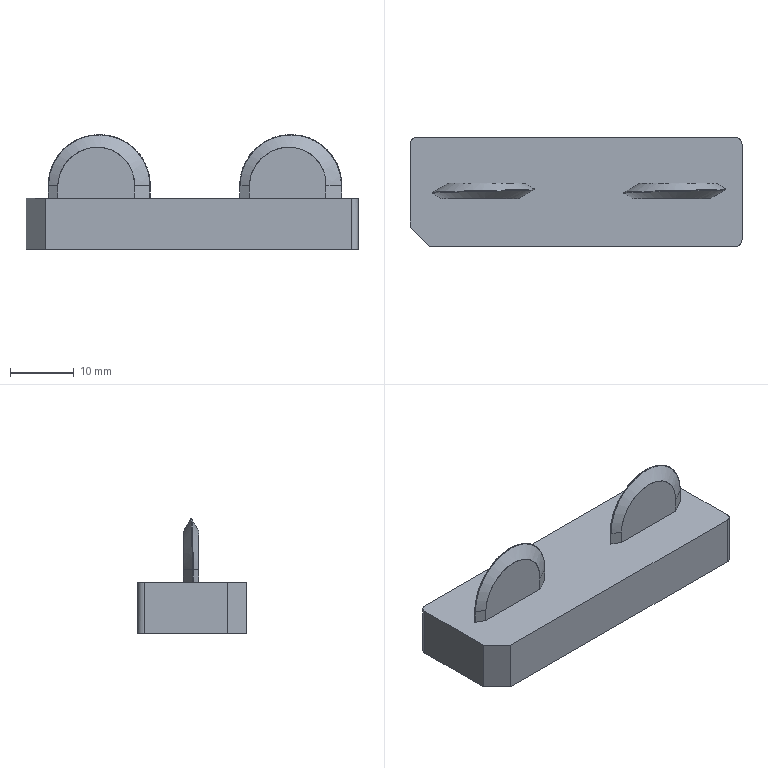NC program | PowerMill | posted with a generic post | part box 52 x 17 x 17.993 mm
Lines 10241 to 10969 of 175197:
N10338 M6
N10339 S18000 M03
N10340 G00 G90 X0.0 Y0.0
N10341 G43 Z10.802 H4
N10342
N10343 G05 P10000 R8
N10344 X-8.3293 Y-0.1432
N10345 Z-1.5814
N10346 G01 Z-2.7814 F1200.0
N10347 X-8.3275 Y-0.123 Z-2.802 F2000.0
N10348 X-8.3219 Y-0.1023 Z-2.8212
N10349 X-8.3129 Y-0.0816 Z-2.8384
N10350 X-8.3006 Y-0.0614 Z-2.8535
N10351 X-8.2852 Y-0.0419 Z-2.8662
N10352 X-8.2758 Y-0.032 Z-2.872
N10353 X-8.235 Y0.0088 Z-2.8945
N10354 X-8.1927 Y0.0511 Z-2.922
N10355 X-8.1485 Y0.0954 Z-2.955
N10356 X-8.1476 Y0.0962 Z-2.9557
N10357 X-8.1288 Y0.1132 Z-2.9682
N10358 X-8.1075 Y0.1291 Z-2.9777
N10359 X-8.0841 Y0.1435 Z-2.9842
N10360 X-8.0591 Y0.1563 Z-2.9874
N10361 X-8.033 Y0.1671
N10362 X-8.0181 Y0.1721 Z-2.9859
N10363 X-7.9685 Y0.2693 Z-3.0277
N10364 X-7.9946 Y0.2585 Z-3.0287
N10365 X-8.0198 Y0.246 Z-3.0263
N10366 X-8.0436 Y0.232 Z-3.0204
N10367 X-8.0655 Y0.2167 Z-3.0112
N10368 X-8.0851 Y0.2006 Z-2.9989
N10369 X-8.095 Y0.1913 Z-2.9908
N10370 X-8.12 Y0.1662 Z-2.9679
N10371 X-8.1518 Y0.1345 Z-2.941
N10372 X-8.1895 Y0.0967 Z-2.9117
N10373 X-8.2367 Y0.0495 Z-2.8782
N10374 X-8.2837 Y0.0026 Z-2.8484
N10375 X-8.3231 Y-0.0368 Z-2.8262
N10376 X-8.3579 Y-0.0716 Z-2.809
N10377 X-8.3933 Y-0.107 Z-2.7944
N10378 X-8.4111 Y-0.1269 Z-2.7853
N10379 X-8.426 Y-0.1479 Z-2.7737
N10380 X-8.4377 Y-0.1696 Z-2.7599
N10381 X-8.4459 Y-0.1915 Z-2.7441
N10382 X-8.4504 Y-0.2133 Z-2.7267
N10383 X-8.4514 Y-0.2252 Z-2.7164
N10384 X-8.5444 Y-0.2776 Z-2.6643
N10385 X-8.5416 Y-0.2552 Z-2.6813
N10386 X-8.535 Y-0.2325 Z-2.6968
N10387 X-8.525 Y-0.2099 Z-2.7104
N10388 X-8.5115 Y-0.188 Z-2.722
N10389 X-8.4951 Y-0.167 Z-2.7313
N10390 X-8.4846 Y-0.1559 Z-2.7354
N10391 X-8.4404 Y-0.1118 Z-2.7505
N10392 X-8.3948 Y-0.0661 Z-2.77
N10393 X-8.3471 Y-0.0184 Z-2.7943
N10394 X-8.2975 Y0.0312 Z-2.8237
N10395 X-8.2464 Y0.0823 Z-2.8582
N10396 X-8.1947 Y0.134 Z-2.8975
N10397 X-8.144 Y0.1847 Z-2.9403
N10398 X-8.097 Y0.2317 Z-2.9841
N10399 X-8.0804 Y0.2482 Z-3.0005
N10400 X-8.0627 Y0.2644 Z-3.0153
N10401 X-8.0424 Y0.2801 Z-3.0271
N10402 X-8.0199 Y0.2948 Z-3.0356
N10403 X-7.9957 Y0.3084 Z-3.0408
N10404 X-7.9703 Y0.3206 Z-3.0424
N10405 X-7.9557 Y0.3267 Z-3.0418
N10406 X-7.9564 Y0.371 Z-3.0433
N10407 X-7.982 Y0.3592 Z-3.0434
N10408 X-8.0067 Y0.3459 Z-3.0399
N10409 X-8.0299 Y0.3315 Z-3.0328
N10410 X-8.0513 Y0.3162 Z-3.0224
N10411 X-8.0703 Y0.3004 Z-3.0088
N10412 X-8.0797 Y0.2914 Z-2.9999
N10413 X-8.1111 Y0.2601 Z-2.9675
N10414 X-8.1603 Y0.2108 Z-2.9201
N10415 X-8.2121 Y0.1591 Z-2.8749
N10416 X-8.2643 Y0.1068 Z-2.8337
N10417 X-8.3161 Y0.055 Z-2.7971
N10418 X-8.3667 Y0.0044 Z-2.7656
N10419 X-8.416 Y-0.0449 Z-2.7389
N10420 X-8.4637 Y-0.0926 Z-2.7171
N10421 X-8.5098 Y-0.1386 Z-2.6998
N10422 X-8.5543 Y-0.1832 Z-2.687
N10423 X-8.5726 Y-0.2036 Z-2.68
N10424 X-8.588 Y-0.2253 Z-2.6707
N10425 X-8.6002 Y-0.248 Z-2.6591
N10426 X-8.609 Y-0.2711 Z-2.6455
N10427 X-8.6143 Y-0.2942 Z-2.6302
N10428 X-8.6156 Y-0.307 Z-2.621
N10429 X-8.6837 Y-0.3327 Z-2.583
N10430 X-8.68 Y-0.3093 Z-2.5983
N10431 X-8.6728 Y-0.2857 Z-2.6119
N10432 X-8.662 Y-0.2623 Z-2.6235
N10433 X-8.648 Y-0.2397 Z-2.6329
N10434 X-8.6311 Y-0.2182 Z-2.64
N10435 X-8.6204 Y-0.2069 Z-2.6428
N10436 X-8.5788 Y-0.1652 Z-2.6521
N10437 X-8.5355 Y-0.122 Z-2.6655
N10438 X-8.4902 Y-0.0767 Z-2.6835
N10439 X-8.4428 Y-0.0293 Z-2.7061
N10440 X-8.3934 Y0.0202 Z-2.7338
N10441 X-8.3421 Y0.0715 Z-2.7667
N10442 X-8.2894 Y0.1241 Z-2.8047
N10443 X-8.2365 Y0.1771 Z-2.8473
N10444 X-8.1856 Y0.228 Z-2.8926
N10445 X-8.1387 Y0.2748 Z-2.9381
N10446 X-8.0965 Y0.317 Z-2.9826
N10447 X-8.0855 Y0.328 Z-2.9949
N10448 X-8.0684 Y0.3437 Z-3.0109
N10449 X-8.0488 Y0.3593 Z-3.0239
N10450 X-8.0269 Y0.3743 Z-3.0336
N10451 X-8.0034 Y0.3886 Z-3.0398
N10452 X-7.9785 Y0.4017 Z-3.0423
N10453 X-7.9643 Y0.4085 Z-3.0422
N10454 X-7.9748 Y0.4434 Z-3.0362
N10455 X-7.9998 Y0.4303 Z-3.0356
N10456 X-8.0238 Y0.4162 Z-3.0313
N10457 X-8.0464 Y0.4012 Z-3.0233
N10458 X-8.0671 Y0.3857 Z-3.0119
N10459 X-8.0855 Y0.3701 Z-2.9973
N10460 X-8.0946 Y0.3614 Z-2.9878
N10461 X-8.1104 Y0.3456 Z-2.9698
N10462 X-8.153 Y0.3029 Z-2.9235
N10463 X-8.2003 Y0.2557 Z-2.8761
N10464 X-8.2515 Y0.2044 Z-2.8289
N10465 X-8.3049 Y0.1511 Z-2.7843
N10466 X-8.3581 Y0.0979 Z-2.7441
N10467 X-8.4102 Y0.0458 Z-2.7089
N10468 X-8.4607 Y-0.0047 Z-2.679
N10469 X-8.5093 Y-0.0534 Z-2.6541
N10470 X-8.5561 Y-0.1001 Z-2.634
N10471 X-8.601 Y-0.145 Z-2.6184
N10472 X-8.644 Y-0.188 Z-2.6073
N10473 X-8.6854 Y-0.2294 Z-2.6003
N10474 X-8.7039 Y-0.2501 Z-2.5956
N10475 X-8.7198 Y-0.2724 Z-2.5886
N10476 X-8.7326 Y-0.2957 Z-2.5791
N10477 X-8.7421 Y-0.3196 Z-2.5676
N10478 X-8.7481 Y-0.3437 Z-2.5541
N10479 X-8.7499 Y-0.3571 Z-2.5458
N10480 X-8.8128 Y-0.3782 Z-2.5117
N10481 X-8.8085 Y-0.3537 Z-2.5251
N10482 X-8.8006 Y-0.3292 Z-2.5366
N10483 X-8.7894 Y-0.305 Z-2.546
N10484 X-8.775 Y-0.2818 Z-2.5531
N10485 X-8.7577 Y-0.26 Z-2.5578
N10486 X-8.7469 Y-0.2485 Z-2.5594
N10487 X-8.714 Y-0.2156 Z-2.5628
N10488 X-8.6799 Y-0.1816 Z-2.5695
N10489 X-8.6408 Y-0.1424 Z-2.5803
N10490 X-8.5955 Y-0.0971 Z-2.5962
N10491 X-8.5466 Y-0.0482 Z-2.6171
N10492 X-8.5059 Y-0.0075 Z-2.6373
N10493 X-8.4721 Y0.0262 Z-2.6561
N10494 X-8.4418 Y0.0566 Z-2.6749
N10495 X-8.3885 Y0.1099 Z-2.7115
N10496 X-8.3346 Y0.1638 Z-2.753
N10497 X-8.2801 Y0.2183 Z-2.7994
N10498 X-8.2257 Y0.2727 Z-2.8503
N10499 X-8.1721 Y0.3263 Z-2.9051
N10500 X-8.1206 Y0.3778 Z-2.9626
N10501 X-8.106 Y0.3924 Z-2.9798
N10502 X-8.0893 Y0.4078 Z-2.9965
N10503 X-8.07 Y0.4232 Z-3.0101
N10504 X-8.0485 Y0.4384 Z-3.0205
N10505 X-8.0253 Y0.4529 Z-3.0272
N10506 X-8.0007 Y0.4665 Z-3.0304
N10507 X-7.9866 Y0.4737 Z-3.0305
N10508 X-8.0003 Y0.5045 Z-3.0226
N10509 X-8.0251 Y0.4911 Z-3.0216
N10510 X-8.0489 Y0.4767 Z-3.0169
N10511 X-8.0713 Y0.4616 Z-3.0085
N10512 X-8.0917 Y0.4462 Z-2.9966
N10513 X-8.1098 Y0.4306 Z-2.9816
N10514 X-8.1188 Y0.422 Z-2.9718
N10515 X-8.1632 Y0.3777 Z-2.9189
N10516 X-8.2114 Y0.3294 Z-2.8658
N10517 X-8.2661 Y0.2747 Z-2.8103
N10518 X-8.3181 Y0.2227 Z-2.7617
N10519 X-8.3704 Y0.1705 Z-2.7169
N10520 X-8.4067 Y0.1342 Z-2.6883
N10521 X-8.4475 Y0.0933 Z-2.6591
N10522 X-8.4939 Y0.0469 Z-2.6292
N10523 X-8.5451 Y-0.0043 Z-2.6
N10524 X-8.5962 Y-0.0554 Z-2.5749
N10525 X-8.6446 Y-0.1038 Z-2.5548
N10526 X-8.6897 Y-0.1489 Z-2.5398
N10527 X-8.7316 Y-0.1908 Z-2.5292
N10528 X-8.7704 Y-0.2295 Z-2.5229
N10529 X-8.8071 Y-0.2663 Z-2.5203
N10530 X-8.8259 Y-0.2872 Z-2.5176
N10531 X-8.842 Y-0.3098 Z-2.5124
N10532 X-8.8552 Y-0.3336 Z-2.5049
N10533 X-8.8652 Y-0.3581 Z-2.4951
N10534 X-8.8718 Y-0.3829 Z-2.4832
N10535 X-8.8739 Y-0.3967 Z-2.4758
N10536 X-8.9331 Y-0.4139 Z-2.4406
N10537 X-8.9284 Y-0.389 Z-2.453
N10538 X-8.9203 Y-0.3641 Z-2.4635
N10539 X-8.9088 Y-0.3397 Z-2.4719
N10540 X-8.8942 Y-0.3163 Z-2.4779
N10541 X-8.8769 Y-0.2943 Z-2.4815
N10542 X-8.8661 Y-0.2828 Z-2.4824
N10543 X-8.8245 Y-0.2413 Z-2.4844
N10544 X-8.782 Y-0.1987 Z-2.4903
N10545 X-8.738 Y-0.1547 Z-2.5003
N10546 X-8.6924 Y-0.1091 Z-2.5147
N10547 X-8.6449 Y-0.0616 Z-2.5336
N10548 X-8.595 Y-0.0117 Z-2.5575
N10549 X-8.5546 Y0.0286 Z-2.5796
N10550 X-8.502 Y0.0813 Z-2.612
N10551 X-8.4491 Y0.1341 Z-2.6489
N10552 X-8.396 Y0.1872 Z-2.6903
N10553 X-8.3427 Y0.2406 Z-2.7365
N10554 X-8.2891 Y0.2941 Z-2.7874
N10555 X-8.2353 Y0.3479 Z-2.8432
N10556 X-8.1814 Y0.4018 Z-2.9041
N10557 X-8.1293 Y0.4539 Z-2.9676
N10558 X-8.1129 Y0.4693 Z-2.9846
N10559 X-8.0939 Y0.4849 Z-2.9985
N10560 X-8.0729 Y0.5005 Z-3.009
N10561 X-8.0501 Y0.5158 Z-3.016
N10562 X-8.0262 Y0.5304 Z-3.0191
N10563 X-8.0124 Y0.5382 Z-3.0192
N10564 X-8.0264 Y0.5669 Z-3.0181
N10565 X-8.0507 Y0.5528 Z-3.0162
N10566 X-8.0741 Y0.5379 Z-3.0106
N10567 X-8.0959 Y0.5226 Z-3.0013
N10568 X-8.1158 Y0.5072 Z-2.9886
N10569 X-8.1333 Y0.492 Z-2.9726
N10570 X-8.1421 Y0.4836 Z-2.9623
N10571 X-8.157 Y0.4687 Z-2.943
N10572 X-8.2099 Y0.4158 Z-2.8779
N10573 X-8.2656 Y0.36 Z-2.8145
N10574 X-8.3071 Y0.3185 Z-2.7705
N10575 X-8.3497 Y0.2759 Z-2.7286
N10576 X-8.3933 Y0.2323 Z-2.6888
N10577 X-8.4462 Y0.1795 Z-2.6443
N10578 X-8.4917 Y0.1339 Z-2.6092
N10579 X-8.5383 Y0.0874 Z-2.5768
N10580 X-8.5882 Y0.0374 Z-2.5458
N10581 X-8.6389 Y-0.0133 Z-2.518
N10582 X-8.6873 Y-0.0616 Z-2.4954
N10583 X-8.7341 Y-0.1084 Z-2.4774
N10584 X-8.7806 Y-0.155 Z-2.4636
N10585 X-8.8277 Y-0.202 Z-2.4536
N10586 X-8.8752 Y-0.2495 Z-2.4477
N10587 X-8.9229 Y-0.2972 Z-2.4457
N10588 X-8.9417 Y-0.3182 Z-2.4436
N10589 X-8.9578 Y-0.3409 Z-2.439
N10590 X-8.9711 Y-0.3648 Z-2.4321
N10591 X-8.9811 Y-0.3896 Z-2.4229
N10592 X-8.9877 Y-0.4146 Z-2.4117
N10593 X-8.9899 Y-0.4286 Z-2.4046
N10594 X-9.0488 Y-0.4451 Z-2.3771
N10595 X-9.0437 Y-0.4197 Z-2.3881
N10596 X-9.0352 Y-0.3943 Z-2.3971
N10597 X-9.0234 Y-0.3695 Z-2.4039
N10598 X-9.0087 Y-0.3459 Z-2.4083
N10599 X-8.9912 Y-0.3238 Z-2.4102
N10600 X-8.9804 Y-0.3123
N10601 X-8.9432 Y-0.2751 Z-2.4088
N10602 X-8.9039 Y-0.2358 Z-2.4111
N10603 X-8.8618 Y-0.1937 Z-2.4173
N10604 X-8.8171 Y-0.149 Z-2.4278
N10605 X-8.7697 Y-0.1016 Z-2.4427
N10606 X-8.7198 Y-0.0517 Z-2.4624
N10607 X-8.6685 Y-0.0004 Z-2.4866
N10608 X-8.6182 Y0.0499 Z-2.5143
N10609 X-8.5722 Y0.0959 Z-2.5431
N10610 X-8.5319 Y0.1362 Z-2.5711
N10611 X-8.479 Y0.1891 Z-2.612
N10612 X-8.426 Y0.2421 Z-2.6573
N10613 X-8.3713 Y0.2968 Z-2.7084
N10614 X-8.3157 Y0.3524 Z-2.7651
N10615 X-8.2606 Y0.4075 Z-2.8261
N10616 X-8.209 Y0.4591 Z-2.888
N10617 X-8.1618 Y0.5063 Z-2.9491
N10618 X-8.1561 Y0.512 Z-2.9568
N10619 X-8.1403 Y0.5268 Z-2.9749
N10620 X-8.122 Y0.5422 Z-2.9899
N10621 X-8.1015 Y0.5577 Z-3.0016
N10622 X-8.0793 Y0.5732 Z-3.0097
N10623 X-8.0558 Y0.5882 Z-3.0141
N10624 X-8.0423 Y0.5964 Z-3.0148
N10625 X-8.0598 Y0.6245 Z-3.0064
N10626 X-8.0834 Y0.6091 Z-3.0043
N10627 X-8.1061 Y0.5934 Z-2.9985
N10628 X-8.1273 Y0.5774 Z-2.9889
N10629 X-8.1467 Y0.5617 Z-2.9758
N10630 X-8.1639 Y0.5464 Z-2.9594
N10631 X-8.1724 Y0.5381 Z-2.9489
N10632 X-8.2011 Y0.5095 Z-2.9102
N10633 X-8.2545 Y0.456 Z-2.842
N10634 X-8.309 Y0.4015 Z-2.7778
N10635 X-8.3639 Y0.3466 Z-2.7181
N10636 X-8.4188 Y0.2917 Z-2.6632
N10637 X-8.4733 Y0.2372 Z-2.6133
N10638 X-8.5273 Y0.1832 Z-2.5684
N10639 X-8.5807 Y0.1298 Z-2.5284
N10640 X-8.6178 Y0.0927 Z-2.5032
N10641 X-8.6675 Y0.043 Z-2.4728
N10642 X-8.7186 Y-0.0081 Z-2.4455
N10643 X-8.7692 Y-0.0587 Z-2.4223
N10644 X-8.8184 Y-0.1079 Z-2.4038
N10645 X-8.8658 Y-0.1552 Z-2.3897
N10646 X-8.9111 Y-0.2006 Z-2.3801
N10647 X-8.9544 Y-0.2439 Z-2.3746
N10648 X-8.9957 Y-0.2851 Z-2.373
N10649 X-9.035 Y-0.3244 Z-2.3753
N10650 X-9.0538 Y-0.3455 Z-2.3751
N10651 X-9.0701 Y-0.3683 Z-2.3725
N10652 X-9.0836 Y-0.3926 Z-2.3675
N10653 X-9.094 Y-0.4178 Z-2.3602
N10654 X-9.1011 Y-0.4434 Z-2.3506
N10655 X-9.1036 Y-0.4577 Z-2.3444
N10656 X-9.1582 Y-0.4699 Z-2.3159
N10657 X-9.1527 Y-0.444 Z-2.3257
N10658 X-9.1439 Y-0.4183 Z-2.3334
N10659 X-9.132 Y-0.3933 Z-2.3388
N10660 X-9.1171 Y-0.3695 Z-2.3417
N10661 X-9.0996 Y-0.3473 Z-2.3422
N10662 X-9.0888 Y-0.3358 Z-2.3413
N10663 X-9.0582 Y-0.3053 Z-2.3379
N10664 X-9.0266 Y-0.2737 Z-2.3374
N10665 X-8.9897 Y-0.2368 Z-2.3398
N10666 X-8.9464 Y-0.1935 Z-2.3459
N10667 X-8.8997 Y-0.1467 Z-2.3561
N10668 X-8.8604 Y-0.1074 Z-2.3674
N10669 X-8.8272 Y-0.0742 Z-2.3792
N10670 X-8.7777 Y-0.0248 Z-2.4004
N10671 X-8.727 Y0.0259 Z-2.4261
N10672 X-8.6746 Y0.0784 Z-2.4567
N10673 X-8.6208 Y0.1322 Z-2.4923
N10674 X-8.5662 Y0.1867 Z-2.5328
N10675 X-8.5119 Y0.241 Z-2.5775
N10676 X-8.4596 Y0.2933 Z-2.625
N10677 X-8.4091 Y0.3438 Z-2.6751
N10678 X-8.353 Y0.3999 Z-2.7353
N10679 X-8.2975 Y0.4555 Z-2.7998
N10680 X-8.2429 Y0.51 Z-2.8684
N10681 X-8.19 Y0.5629 Z-2.9401
N10682 X-8.189 Y0.5639 Z-2.9415
N10683 X-8.1735 Y0.5785 Z-2.9601
N10684 X-8.1556 Y0.5937 Z-2.9756
N10685 X-8.1354 Y0.6093 Z-2.9878
N10686 X-8.1136 Y0.625 Z-2.9964
N10687 X-8.0904 Y0.6404 Z-3.0012
N10688 X-8.077 Y0.6488 Z-3.0022
N10689 X-8.1 Y0.6716 Z-2.9892
N10690 X-8.1233 Y0.6558 Z-2.9867
N10691 X-8.1456 Y0.6398 Z-2.9803
N10692 X-8.1665 Y0.6237 Z-2.9702
N10693 X-8.1855 Y0.6079 Z-2.9566
N10694 X-8.2024 Y0.5928 Z-2.9397
N10695 X-8.2107 Y0.5847 Z-2.929
N10696 X-8.243 Y0.5524 Z-2.8834
N10697 X-8.2938 Y0.5016 Z-2.8159
N10698 X-8.347 Y0.4483 Z-2.7503
N10699 X-8.4016 Y0.3938 Z-2.6881
N10700 X-8.4567 Y0.3387 Z-2.6301
N10701 X-8.5119 Y0.2835 Z-2.5769
N10702 X-8.5667 Y0.2287 Z-2.5285
N10703 X-8.621 Y0.1744 Z-2.4852
N10704 X-8.6746 Y0.1208 Z-2.4467
N10705 X-8.7273 Y0.0681 Z-2.4131
N10706 X-8.7792 Y0.0162 Z-2.3841
N10707 X-8.8301 Y-0.0347 Z-2.3598
N10708 X-8.8801 Y-0.0848 Z-2.3398
N10709 X-8.9284 Y-0.1331 Z-2.3243
N10710 X-8.9752 Y-0.1799 Z-2.3129
N10711 X-9.0197 Y-0.2243 Z-2.3058
N10712 X-9.0622 Y-0.2668 Z-2.3027
N10713 X-9.1029 Y-0.3075 Z-2.3035
N10714 X-9.1422 Y-0.3469 Z-2.308
N10715 X-9.161 Y-0.3679 Z-2.3091
N10716 X-9.1774 Y-0.3908 Z-2.3076
N10717 X-9.191 Y-0.4152 Z-2.3037
N10718 X-9.2016 Y-0.4406 Z-2.2974
N10719 X-9.209 Y-0.4665 Z-2.2889
N10720 X-9.2116 Y-0.481 Z-2.2831
N10721 X-9.2663 Y-0.493 Z-2.2518
N10722 X-9.2607 Y-0.467 Z-2.2614
N10723 X-9.2518 Y-0.4413 Z-2.2687
N10724 X-9.2398 Y-0.4162 Z-2.2737
N10725 X-9.2249 Y-0.3924 Z-2.2763
N10726 X-9.2074 Y-0.3702
N10727 X-9.1966 Y-0.3588 Z-2.2752
N10728 X-9.1559 Y-0.3181 Z-2.2698
N10729 X-9.114 Y-0.2762 Z-2.2682
N10730 X-9.0705 Y-0.2327 Z-2.2704
N10731 X-9.0254 Y-0.1876 Z-2.2766
N10732 X-8.9786 Y-0.1408 Z-2.287
N10733 X-8.9301 Y-0.0923 Z-2.3018
N10734 X-8.8798 Y-0.042 Z-2.321
N10735 X-8.8279 Y0.0099 Z-2.3449
N10736 X-8.7757 Y0.0621 Z-2.3731
N10737 X-8.723 Y0.1148 Z-2.4057
N10738 X-8.6699 Y0.1679 Z-2.4429
N10739 X-8.6163 Y0.2215 Z-2.4847
N10740 X-8.561 Y0.2768 Z-2.5323
N10741 X-8.5058 Y0.332 Z-2.5844
N10742 X-8.4507 Y0.3871 Z-2.6411
N10743 X-8.3959 Y0.4419 Z-2.7025
N10744 X-8.3413 Y0.4965 Z-2.7686
N10745 X-8.2883 Y0.5495 Z-2.8376
N10746 X-8.2391 Y0.5987 Z-2.9067
N10747 X-8.2344 Y0.6034 Z-2.9136
N10748 X-8.2192 Y0.6178 Z-2.9326
N10749 X-8.2016 Y0.6331 Z-2.9485
N10750 X-8.1819 Y0.6489 Z-2.9611
N10751 X-8.1605 Y0.665 Z-2.9701
N10752 X-8.1379 Y0.681 Z-2.9753
N10753 X-8.1248 Y0.6899 Z-2.9765
N10754 X-8.1498 Y0.7104 Z-2.9605
N10755 X-8.1725 Y0.6939 Z-2.9578
N10756 X-8.1944 Y0.6773 Z-2.9511
N10757 X-8.2149 Y0.6609 Z-2.9407
N10758 X-8.2336 Y0.645 Z-2.9268
N10759 X-8.2501 Y0.6299 Z-2.9096
N10760 X-8.2583 Y0.6219 Z-2.8987
N10761 X-8.2911 Y0.5891 Z-2.851
N10762 X-8.3422 Y0.538 Z-2.7811
N10763 X-8.3967 Y0.4836 Z-2.7122
N10764 X-8.4522 Y0.428 Z-2.647
N10765 X-8.5076 Y0.3726 Z-2.5869
N10766 X-8.562 Y0.3182 Z-2.5326
N10767 X-8.6157 Y0.2645 Z-2.4833
N10768 X-8.6699 Y0.2103 Z-2.4382
N10769 X-8.7242 Y0.156 Z-2.3975
N10770 X-8.7786 Y0.1016 Z-2.3611
N10771 X-8.8331 Y0.0471 Z-2.3289
N10772 X-8.8839 Y-0.0037 Z-2.3028
N10773 X-8.9347 Y-0.0545 Z-2.2807
N10774 X-8.9846 Y-0.1044 Z-2.2629
N10775 X-9.0331 Y-0.1529 Z-2.2495
N10776 X-9.0799 Y-0.1997 Z-2.2404
N10777 X-9.1249 Y-0.2446 Z-2.2354
N10778 X-9.1679 Y-0.2877 Z-2.2343
N10779 X-9.2091 Y-0.3289 Z-2.2371
N10780 X-9.2484 Y-0.3682 Z-2.2434
N10781 X-9.2672 Y-0.3892 Z-2.2454
N10782 X-9.2836 Y-0.4121 Z-2.2449
N10783 X-9.2973 Y-0.4366 Z-2.2418
N10784 X-9.3081 Y-0.4621 Z-2.2363
N10785 X-9.3156 Y-0.4882 Z-2.2285
N10786 X-9.3184 Y-0.5028 Z-2.2231
N10787 X-9.3709 Y-0.5128 Z-2.195
N10788 X-9.3651 Y-0.4865 Z-2.2036
N10789 X-9.356 Y-0.4606 Z-2.21
N10790 X-9.3438 Y-0.4354 Z-2.2139
N10791 X-9.3288 Y-0.4115 Z-2.2153
N10792 X-9.3114 Y-0.3894 Z-2.2141
N10793 X-9.3006 Y-0.3779 Z-2.2124
N10794 X-9.2623 Y-0.3396 Z-2.2051
N10795 X-9.2218 Y-0.2992 Z-2.2013
N10796 X-9.1793 Y-0.2567 Z-2.2012
N10797 X-9.1347 Y-0.212 Z-2.2049
N10798 X-9.0879 Y-0.1653 Z-2.2128
N10799 X-9.0393 Y-0.1167 Z-2.2249
N10800 X-8.9892 Y-0.0665 Z-2.2413
N10801 X-8.9382 Y-0.0155 Z-2.262
N10802 X-8.8876 Y0.0351 Z-2.2865
N10803 X-8.8397 Y0.083 Z-2.3134
N10804 X-8.7976 Y0.1251 Z-2.34
N10805 X-8.7468 Y0.1758 Z-2.3756
N10806 X-8.692 Y0.2307 Z-2.4179
N10807 X-8.6413 Y0.2813 Z-2.4607
N10808 X-8.5938 Y0.3288 Z-2.5044
N10809 X-8.5476 Y0.3751 Z-2.5507
N10810 X-8.4953 Y0.4274 Z-2.6071
N10811 X-8.4411 Y0.4815 Z-2.6701
N10812 X-8.3861 Y0.5366 Z-2.7391
N10813 X-8.3371 Y0.5855 Z-2.8049
N10814 X-8.2911 Y0.6315 Z-2.8713
N10815 X-8.2826 Y0.64 Z-2.8842
N10816 X-8.2677 Y0.6543 Z-2.9034
N10817 X-8.2503 Y0.6695 Z-2.9196
N10818 X-8.2309 Y0.6855 Z-2.9325
N10819 X-8.2099 Y0.7018 Z-2.9418
N10820 X-8.1876 Y0.7182 Z-2.9473
N10821 X-8.1747 Y0.7273 Z-2.9487
N10822 X-8.2012 Y0.7468 Z-2.9316
N10823 X-8.2235 Y0.7298 Z-2.9286
N10824 X-8.245 Y0.7128 Z-2.9217
N10825 X-8.2651 Y0.6962 Z-2.9111
N10826 X-8.2835 Y0.6801 Z-2.8969
N10827 X-8.2998 Y0.6651 Z-2.8794
N10828 X-8.3079 Y0.6571 Z-2.8684
N10829 X-8.3412 Y0.6239 Z-2.8187
N10830 X-8.3921 Y0.573 Z-2.7472
N10831 X-8.4453 Y0.5198 Z-2.6777
N10832 X-8.4998 Y0.4653 Z-2.6116
N10833 X-8.5551 Y0.41 Z-2.5496
N10834 X-8.6107 Y0.3544 Z-2.4921
N10835 X-8.6662 Y0.2988 Z-2.4395
N10836 X-8.7215 Y0.2436 Z-2.3917
N10837 X-8.7762 Y0.1888 Z-2.3488
N10838 X-8.8304 Y0.1347 Z-2.3107
N10839 X-8.884 Y0.0811 Z-2.2772
N10840 X-8.9368 Y0.0283 Z-2.2484
N10841 X-8.989 Y-0.0239 Z-2.224
N10842 X-9.0404 Y-0.0753 Z-2.204
N10843 X-9.0903 Y-0.1252 Z-2.1885
N10844 X-9.1382 Y-0.1731 Z-2.1774
N10845 X-9.1843 Y-0.2192 Z-2.1705
N10846 X-9.2287 Y-0.2636 Z-2.1676
N10847 X-9.2714 Y-0.3063 Z-2.1687
N10848 X-9.3127 Y-0.3476 Z-2.1734
N10849 X-9.3526 Y-0.3875 Z-2.1819
N10850 X-9.3713 Y-0.4084 Z-2.1848
N10851 X-9.3877 Y-0.4314 Z-2.1852
N10852 X-9.4015 Y-0.4559 Z-2.1831
N10853 X-9.4123 Y-0.4816 Z-2.1786
N10854 X-9.42 Y-0.5078 Z-2.1716
N10855 X-9.4229 Y-0.5226 Z-2.1667
N10856 X-9.4743 Y-0.5313 Z-2.1397
N10857 X-9.4683 Y-0.5048 Z-2.1476
N10858 X-9.459 Y-0.4787 Z-2.1531
N10859 X-9.4468 Y-0.4535 Z-2.1561
N10860 X-9.4318 Y-0.4296 Z-2.1565
N10861 X-9.4143 Y-0.4075 Z-2.1545
N10862 X-9.4036 Y-0.3961 Z-2.1522
N10863 X-9.3654 Y-0.3579 Z-2.143
N10864 X-9.3252 Y-0.3177 Z-2.1372
N10865 X-9.283 Y-0.2755 Z-2.1351
N10866 X-9.2387 Y-0.2312 Z-2.1368
N10867 X-9.1924 Y-0.1849 Z-2.1425
N10868 X-9.1443 Y-0.1367 Z-2.1524
N10869 X-9.0944 Y-0.0869 Z-2.1665
N10870 X-9.0435 Y-0.036 Z-2.185
N10871 X-8.9924 Y0.0151 Z-2.2074
N10872 X-8.9428 Y0.0647 Z-2.2329
N10873 X-8.8947 Y0.1128 Z-2.2612
N10874 X-8.8412 Y0.1663 Z-2.2967
N10875 X-8.7869 Y0.2206 Z-2.3371
N10876 X-8.7319 Y0.2756 Z-2.3824
N10877 X-8.6762 Y0.3313 Z-2.4327
N10878 X-8.6203 Y0.3872 Z-2.488
N10879 X-8.5643 Y0.4432 Z-2.5481
N10880 X-8.5089 Y0.4986 Z-2.6127
N10881 X-8.4545 Y0.553 Z-2.681
N10882 X-8.4019 Y0.6056 Z-2.7522
N10883 X-8.3524 Y0.6551 Z-2.8244
N10884 X-8.3349 Y0.6727 Z-2.8512
N10885 X-8.32 Y0.6869 Z-2.8706
N10886 X-8.3029 Y0.7023 Z-2.8869
N10887 X-8.2838 Y0.7185 Z-2.8999
N10888 X-8.2631 Y0.7353 Z-2.9093
N10889 X-8.2412 Y0.7522 Z-2.9148
N10890 X-8.2286 Y0.7617 Z-2.9162
N10891 X-8.2578 Y0.7783 Z-2.8967
N10892 X-8.2797 Y0.7608 Z-2.8935
N10893 X-8.3007 Y0.7434 Z-2.8864
N10894 X-8.3205 Y0.7264 Z-2.8756
N10895 X-8.3386 Y0.7102 Z-2.8612
N10896 X-8.3547 Y0.6951 Z-2.8436
N10897 X-8.3627 Y0.6873 Z-2.8324
N10898 X-8.3892 Y0.6607 Z-2.792
N10899 X-8.4431 Y0.6069 Z-2.7143
N10900 X-8.4974 Y0.5526 Z-2.6413
N10901 X-8.5521 Y0.4978 Z-2.5731
N10902 X-8.6072 Y0.4427 Z-2.5095
N10903 X-8.6627 Y0.3872 Z-2.4505
N10904 X-8.7185 Y0.3315 Z-2.396
N10905 X-8.7746 Y0.2754 Z-2.346
N10906 X-8.8267 Y0.2232 Z-2.3035
N10907 X-8.881 Y0.1689 Z-2.2637
N10908 X-8.9359 Y0.114 Z-2.2278
N10909 X-8.9904 Y0.0595 Z-2.1964
N10910 X-9.0438 Y0.0061 Z-2.1697
N10911 X-9.0956 Y-0.0457 Z-2.1478
N10912 X-9.1457 Y-0.0958 Z-2.1304
N10913 X-9.1938 Y-0.1439 Z-2.1174
N10914 X-9.24 Y-0.1901 Z-2.1087
N10915 X-9.2854 Y-0.2354 Z-2.1038
N10916 X-9.3299 Y-0.2799 Z-2.1029
N10917 X-9.3728 Y-0.3229 Z-2.1058
N10918 X-9.4141 Y-0.3642 Z-2.1124
N10919 X-9.4539 Y-0.4039 Z-2.1226
N10920 X-9.4725 Y-0.4248 Z-2.1264
N10921 X-9.4889 Y-0.4477 Z-2.1276
N10922 X-9.5027 Y-0.4723 Z-2.1263
N10923 X-9.5137 Y-0.498 Z-2.1225
N10924 X-9.5216 Y-0.5244 Z-2.1162
N10925 X-9.5246 Y-0.5392 Z-2.1117
N10926 X-9.5749 Y-0.5473 Z-2.0905
N10927 X-9.5686 Y-0.5206 Z-2.0967
N10928 X-9.5592 Y-0.4942 Z-2.1005
N10929 X-9.5469 Y-0.4688 Z-2.1018
N10930 X-9.5319 Y-0.4449 Z-2.1004
N10931 X-9.5146 Y-0.423 Z-2.0965
N10932 X-9.504 Y-0.4117 Z-2.0932
N10933 X-9.5 Y-0.4076 Z-2.0918
N10934 X-9.4594 Y-0.367 Z-2.0812
N10935 X-9.4176 Y-0.3253 Z-2.0744
N10936 X-9.3745 Y-0.2821 Z-2.0712
N10937 X-9.3299 Y-0.2375 Z-2.0718
N10938 X-9.2838 Y-0.1914 Z-2.0764
N10939 X-9.236 Y-0.1437 Z-2.0851
N10940 X-9.1866 Y-0.0943 Z-2.0981
N10941 X-9.1355 Y-0.0432 Z-2.1154
N10942 X-9.0891 Y0.0033 Z-2.1345
N10943 X-9.0403 Y0.0521 Z-2.1582
N10944 X-8.9899 Y0.1025 Z-2.1866
N10945 X-8.9362 Y0.1561 Z-2.2207
N10946 X-8.88 Y0.2123 Z-2.2607
N10947 X-8.8235 Y0.2689 Z-2.3052
N10948 X-8.7715 Y0.3209 Z-2.3502
N10949 X-8.725 Y0.3673 Z-2.3938
N10950 X-8.6817 Y0.4106 Z-2.4377
N10951 X-8.6314 Y0.461 Z-2.4927
N10952 X-8.5792 Y0.5132 Z-2.554
N10953 X-8.5233 Y0.569 Z-2.6244
N10954 X-8.4729 Y0.6194 Z-2.6925
N10955 X-8.4285 Y0.6639 Z-2.7569
N10956 X-8.3911 Y0.7013 Z-2.8146
N10957 X-8.3764 Y0.7155 Z-2.834
N10958 X-8.3595 Y0.731 Z-2.8504
N10959 X-8.3406 Y0.7475 Z-2.8634
N10960 X-8.3203 Y0.7646 Z-2.8729
N10961 X-8.2988 Y0.7821 Z-2.8785
N10962 X-8.2864 Y0.7919 Z-2.8799
N10963 X-8.3165 Y0.8044 Z-2.8613
N10964 X-8.3384 Y0.7869 Z-2.8577
N10965 X-8.3594 Y0.7696 Z-2.8501
N10966 X-8.379 Y0.7527 Z-2.8388
N10967 X-8.3969 Y0.7367 Z-2.824
N10968 X-8.4128 Y0.7218 Z-2.806
N10969 X-8.4207 Y0.7141 Z-2.7947
N10970 X-8.4429 Y0.6918 Z-2.7596
N10971 X-8.4922 Y0.6426 Z-2.6861
N10972 X-8.5446 Y0.5902 Z-2.6136
N10973 X-8.5991 Y0.5356 Z-2.5436
N10974 X-8.6549 Y0.4799 Z-2.4774
N10975 X-8.711 Y0.4238 Z-2.4156
N10976 X-8.7671 Y0.3676 Z-2.3588
N10977 X-8.8228 Y0.312 Z-2.3071
N10978 X-8.8778 Y0.257 Z-2.2603
N10979 X-8.933 Y0.2018 Z-2.2179
N10980 X-8.9875 Y0.1473 Z-2.1803
N10981 X-9.0413 Y0.0935 Z-2.1474
N10982 X-9.0944 Y0.0404 Z-2.1191
N10983 X-9.1468 Y-0.0121 Z-2.0952
N10984 X-9.1986 Y-0.0639 Z-2.0757
N10985 X-9.2498 Y-0.115 Z-2.0604
N10986 X-9.2998 Y-0.165 Z-2.0493
N10987 X-9.347 Y-0.2122 Z-2.0423
N10988 X-9.3916 Y-0.2568 Z-2.0394
N10989 X-9.434 Y-0.2992 Z-2.0403
N10990 X-9.4749 Y-0.3401 Z-2.0449
N10991 X-9.5144 Y-0.3796 Z-2.0531
N10992 X-9.5535 Y-0.4187 Z-2.0648
N10993 X-9.5721 Y-0.4395 Z-2.0694
N10994 X-9.5885 Y-0.4624 Z-2.0715
N10995 X-9.6023 Y-0.487 Z-2.071
N10996 X-9.6134 Y-0.5128 Z-2.0679
N10997 X-9.6214 Y-0.5392 Z-2.0623
N10998 X-9.6246 Y-0.5542 Z-2.0581
N10999 X-9.6753 Y-0.5627 Z-2.0334
N11000 X-9.669 Y-0.536 Z-2.0399
N11001 X-9.6596 Y-0.5096 Z-2.0439
N11002 X-9.6472 Y-0.4843 Z-2.0454
N11003 X-9.6323 Y-0.4604 Z-2.0442
N11004 X-9.6149 Y-0.4384 Z-2.0406
N11005 X-9.6043 Y-0.4271 Z-2.0374
N11006 X-9.5657 Y-0.3885 Z-2.0248
N11007 X-9.5254 Y-0.3482 Z-2.0157
N11008 X-9.4834 Y-0.3062 Z-2.0102
N11009 X-9.4397 Y-0.2624 Z-2.0085
N11010 X-9.3942 Y-0.217 Z-2.0106
N11011 X-9.347 Y-0.1698 Z-2.0167
N11012 X-9.2981 Y-0.1209 Z-2.0269
N11013 X-9.2476 Y-0.0704 Z-2.0415
N11014 X-9.1956 Y-0.0184 Z-2.0605
N11015 X-9.1426 Y0.0346 Z-2.0838
N11016 X-9.0892 Y0.088 Z-2.1114
N11017 X-9.0363 Y0.1409 Z-2.1427
N11018 X-8.9991 Y0.1781 Z-2.1671
N11019 X-8.9447 Y0.2325 Z-2.2065
N11020 X-8.8898 Y0.2874 Z-2.2505
N11021 X-8.8344 Y0.3428 Z-2.2996
N11022 X-8.7785 Y0.3987 Z-2.3536
N11023 X-8.7225 Y0.4547 Z-2.4126
N11024 X-8.6665 Y0.5107 Z-2.4764
N11025 X-8.6111 Y0.5661 Z-2.5446
N11026 X-8.5567 Y0.6205 Z-2.6168
N11027 X-8.5041 Y0.6731 Z-2.6919
N11028 X-8.4542 Y0.723 Z-2.7684
N11029 X-8.4506 Y0.7266 Z-2.7741
N11030 X-8.4362 Y0.7406 Z-2.7939
N11031 X-8.4195 Y0.756 Z-2.8106
N11032 X-8.4008 Y0.7724 Z-2.8241
N11033 X-8.3807 Y0.7896 Z-2.8339
N11034 X-8.3594 Y0.8071 Z-2.8399
N11035 X-8.3471 Y0.817 Z-2.8415
N11036 X-8.3783 Y0.8315 Z-2.8221
N11037 X-8.3996 Y0.8133 Z-2.8185
N11038 X-8.4201 Y0.7954 Z-2.8109
N11039 X-8.4393 Y0.7781 Z-2.7997
N11040 X-8.457 Y0.7618 Z-2.7849
N11041 X-8.4727 Y0.7468 Z-2.7668
N11042 X-8.4805 Y0.7391 Z-2.7555
N11043 X-8.5153 Y0.7043 Z-2.7004
N11044 X-8.5617 Y0.658 Z-2.6315
N11045 X-8.6133 Y0.6064 Z-2.5599
N11046 X-8.669 Y0.5507 Z-2.488
N11047 X-8.7243 Y0.4953 Z-2.4218
N11048 X-8.7776 Y0.442 Z-2.3625
N11049 X-8.8294 Y0.3902 Z-2.3093
N11050 X-8.8737 Y0.346 Z-2.2672
N11051 X-8.9203 Y0.2993 Z-2.2263
N11052 X-8.9735 Y0.2461 Z-2.1835
N11053 X-9.0308 Y0.1889 Z-2.1417
N11054 X-9.0849 Y0.1348 Z-2.1062
N11055 X-9.1347 Y0.085 Z-2.0771
N11056 X-9.1805 Y0.0391 Z-2.0536
N11057 X-9.2341 Y-0.0145 Z-2.03
N11058 X-9.2862 Y-0.0666 Z-2.0109
N11059 X-9.3368 Y-0.1171 Z-1.9963
N11060 X-9.3857 Y-0.166 Z-1.986
N11061 X-9.433 Y-0.2133 Z-1.9799
N11062 X-9.4787 Y-0.2591 Z-1.9777
N11063 X-9.523 Y-0.3034 Z-1.9794
N11064 X-9.5658 Y-0.3461 Z-1.9849
N11065 X-9.6072 Y-0.3875 Z-1.9941
N11066 X-9.6473 Y-0.4277 Z-2.0069